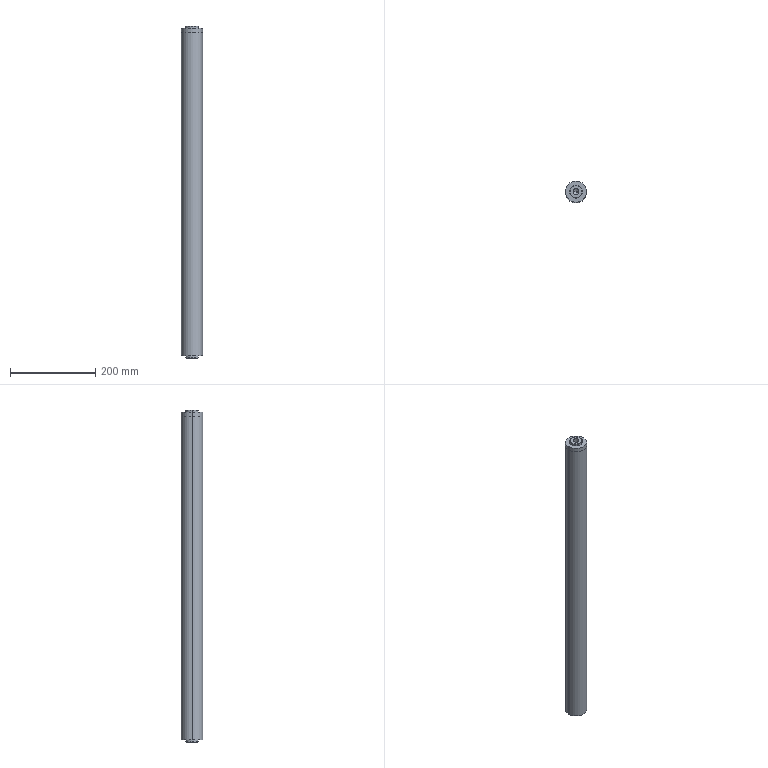Part | STEP file | circular post SPCD-SSB-D50-L760-E5-P30-M16-F15-V30-MA16-SC40-W20-S41 | 2 solids | 28 faces | box 50 x 50 x 780 mm | volume 1506737 mm3 | cylinder 14 | cone 8 | plane 6 | commonest cylinder face diameters 30 x6 14 x4 50 x4